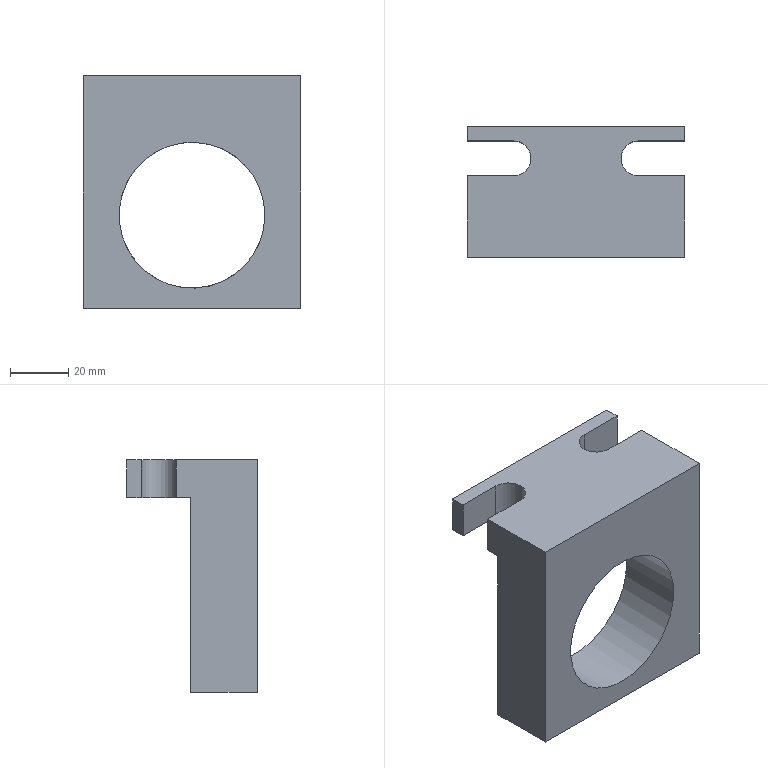Part | NX | features solid 2 | 1 solid | 17 faces | box 75 x 45 x 80 mm | volume 107465 mm3 | plane 14 | cylinder 3 | commonest cylinder face diameters 12 x2 50.2 x1
STEP:
#1=CARTESIAN_POINT('',(297.5,589.4,185.));
#2=VERTEX_POINT('',#1);
#3=CARTESIAN_POINT('',(372.5,589.4,185.));
#4=VERTEX_POINT('',#3);
#5=CARTESIAN_POINT('',(302.5,589.4,185.));
#6=DIRECTION('',(1.,0.,0.));
#7=VECTOR('',#6,1000.);
#8=LINE('',#5,#7);
#9=EDGE_CURVE('',#2,#4,#8,.T.);
#10=ORIENTED_EDGE('',*,*,#9,.F.);
#11=CARTESIAN_POINT('',(297.5,594.4,185.));
#12=VERTEX_POINT('',#11);
#13=CARTESIAN_POINT('',(297.5,565.9,185.));
#14=DIRECTION('',(0.,-1.,0.));
#15=VECTOR('',#14,1000.);
#16=LINE('',#13,#15);
#17=EDGE_CURVE('',#2,#12,#16,.F.);
#18=ORIENTED_EDGE('',*,*,#17,.T.);
#19=CARTESIAN_POINT('',(313.5,594.4,185.));
#20=VERTEX_POINT('',#19);
#21=CARTESIAN_POINT('',(302.5,594.4,185.));
#22=DIRECTION('',(-1.,0.,0.));
#23=VECTOR('',#22,1000.);
#24=LINE('',#21,#23);
#25=EDGE_CURVE('',#12,#20,#24,.F.);
#26=ORIENTED_EDGE('',*,*,#25,.T.);
#27=CARTESIAN_POINT('',(313.5,606.4,185.));
#28=VERTEX_POINT('',#27);
#29=CARTESIAN_POINT('',(313.5,600.4,185.));
#30=DIRECTION('',(0.,0.,-1.));
#31=DIRECTION('',(-1.,0.,0.));
#32=AXIS2_PLACEMENT_3D('',#29,#30,#31);
#33=CIRCLE('',#32,6.);
#34=EDGE_CURVE('',#28,#20,#33,.T.);
#35=ORIENTED_EDGE('',*,*,#34,.F.);
#36=CARTESIAN_POINT('',(297.5,606.4,185.));
#37=VERTEX_POINT('',#36);
#38=CARTESIAN_POINT('',(302.5,606.4,185.));
#39=DIRECTION('',(-1.,0.,0.));
#40=VECTOR('',#39,1000.);
#41=LINE('',#38,#40);
#42=EDGE_CURVE('',#37,#28,#41,.F.);
#43=ORIENTED_EDGE('',*,*,#42,.F.);
#44=CARTESIAN_POINT('',(297.5,611.4,185.));
#45=VERTEX_POINT('',#44);
#46=CARTESIAN_POINT('',(297.5,565.9,185.));
#47=DIRECTION('',(0.,-1.,0.));
#48=VECTOR('',#47,1000.);
#49=LINE('',#46,#48);
#50=EDGE_CURVE('',#37,#45,#49,.F.);
#51=ORIENTED_EDGE('',*,*,#50,.T.);
#52=CARTESIAN_POINT('',(372.5,611.4,185.));
#53=VERTEX_POINT('',#52);
#54=CARTESIAN_POINT('',(302.5,611.4,185.));
#55=DIRECTION('',(-1.,0.,0.));
#56=VECTOR('',#55,1000.);
#57=LINE('',#54,#56);
#58=EDGE_CURVE('',#45,#53,#57,.F.);
#59=ORIENTED_EDGE('',*,*,#58,.T.);
#60=CARTESIAN_POINT('',(372.5,606.4,185.));
#61=VERTEX_POINT('',#60);
#62=CARTESIAN_POINT('',(372.5,565.9,185.));
#63=DIRECTION('',(0.,-1.,0.));
#64=VECTOR('',#63,1000.);
#65=LINE('',#62,#64);
#66=EDGE_CURVE('',#61,#53,#65,.F.);
#67=ORIENTED_EDGE('',*,*,#66,.F.);
#68=CARTESIAN_POINT('',(356.5,606.4,185.));
#69=VERTEX_POINT('',#68);
#70=CARTESIAN_POINT('',(302.5,606.4,185.));
#71=DIRECTION('',(1.,0.,0.));
#72=VECTOR('',#71,1000.);
#73=LINE('',#70,#72);
#74=EDGE_CURVE('',#61,#69,#73,.F.);
#75=ORIENTED_EDGE('',*,*,#74,.T.);
#76=CARTESIAN_POINT('',(356.5,594.4,185.));
#77=VERTEX_POINT('',#76);
#78=CARTESIAN_POINT('',(356.5,600.4,185.));
#79=DIRECTION('',(0.,0.,-1.));
#80=DIRECTION('',(-1.,0.,0.));
#81=AXIS2_PLACEMENT_3D('',#78,#79,#80);
#82=CIRCLE('',#81,6.);
#83=EDGE_CURVE('',#69,#77,#82,.F.);
#84=ORIENTED_EDGE('',*,*,#83,.T.);
#85=CARTESIAN_POINT('',(372.5,594.4,185.));
#86=VERTEX_POINT('',#85);
#87=CARTESIAN_POINT('',(302.5,594.4,185.));
#88=DIRECTION('',(1.,0.,0.));
#89=VECTOR('',#88,1000.);
#90=LINE('',#87,#89);
#91=EDGE_CURVE('',#86,#77,#90,.F.);
#92=ORIENTED_EDGE('',*,*,#91,.F.);
#93=CARTESIAN_POINT('',(372.5,565.9,185.));
#94=DIRECTION('',(0.,-1.,0.));
#95=VECTOR('',#94,1000.);
#96=LINE('',#93,#95);
#97=EDGE_CURVE('',#4,#86,#96,.F.);
#98=ORIENTED_EDGE('',*,*,#97,.F.);
#99=EDGE_LOOP('',(#10,#18,#26,#35,#43,#51,#59,#67,#75,#84,#92,#98));
#100=FACE_BOUND('',#99,.T.);
#101=CARTESIAN_POINT('',(302.5,565.9,185.));
#102=DIRECTION('',(0.,0.,-1.));
#103=DIRECTION('',(1.,0.,0.));
#104=AXIS2_PLACEMENT_3D('',#101,#102,#103);
#105=PLANE('',#104);
#106=ADVANCED_FACE('',(#100),#105,.T.);
#107=CARTESIAN_POINT('',(297.5,611.4,198.));
#108=VERTEX_POINT('',#107);
#109=CARTESIAN_POINT('',(372.5,611.4,198.));
#110=VERTEX_POINT('',#109);
#111=CARTESIAN_POINT('',(302.5,611.4,198.));
#112=DIRECTION('',(-1.,0.,0.));
#113=VECTOR('',#112,1000.);
#114=LINE('',#111,#113);
#115=EDGE_CURVE('',#108,#110,#114,.F.);
#116=ORIENTED_EDGE('',*,*,#115,.T.);
#117=CARTESIAN_POINT('',(372.5,611.4,190.));
#118=DIRECTION('',(0.,0.,1.));
#119=VECTOR('',#118,1000.);
#120=LINE('',#117,#119);
#121=EDGE_CURVE('',#53,#110,#120,.T.);
#122=ORIENTED_EDGE('',*,*,#121,.F.);
#123=ORIENTED_EDGE('',*,*,#58,.F.);
#124=CARTESIAN_POINT('',(297.5,611.4,190.));
#125=DIRECTION('',(0.,0.,1.));
#126=VECTOR('',#125,1000.);
#127=LINE('',#124,#126);
#128=EDGE_CURVE('',#45,#108,#127,.T.);
#129=ORIENTED_EDGE('',*,*,#128,.T.);
#130=EDGE_LOOP('',(#116,#122,#123,#129));
#131=FACE_BOUND('',#130,.T.);
#132=CARTESIAN_POINT('',(302.5,611.4,190.));
#133=DIRECTION('',(0.,-1.,0.));
#134=DIRECTION('',(1.,0.,0.));
#135=AXIS2_PLACEMENT_3D('',#132,#133,#134);
#136=PLANE('',#135);
#137=ADVANCED_FACE('',(#131),#136,.F.);
#138=CARTESIAN_POINT('',(297.5,606.4,198.));
#139=VERTEX_POINT('',#138);
#140=CARTESIAN_POINT('',(297.5,565.9,198.));
#141=DIRECTION('',(0.,-1.,0.));
#142=VECTOR('',#141,1000.);
#143=LINE('',#140,#142);
#144=EDGE_CURVE('',#139,#108,#143,.F.);
#145=ORIENTED_EDGE('',*,*,#144,.T.);
#146=ORIENTED_EDGE('',*,*,#128,.F.);
#147=ORIENTED_EDGE('',*,*,#50,.F.);
#148=CARTESIAN_POINT('',(297.5,606.4,190.));
#149=DIRECTION('',(0.,0.,1.));
#150=VECTOR('',#149,1000.);
#151=LINE('',#148,#150);
#152=EDGE_CURVE('',#37,#139,#151,.T.);
#153=ORIENTED_EDGE('',*,*,#152,.T.);
#154=EDGE_LOOP('',(#145,#146,#147,#153));
#155=FACE_BOUND('',#154,.T.);
#156=CARTESIAN_POINT('',(297.5,565.9,190.));
#157=DIRECTION('',(1.,0.,0.));
#158=DIRECTION('',(0.,1.,0.));
#159=AXIS2_PLACEMENT_3D('',#156,#157,#158);
#160=PLANE('',#159);
#161=ADVANCED_FACE('',(#155),#160,.F.);
#162=CARTESIAN_POINT('',(313.5,606.4,198.));
#163=VERTEX_POINT('',#162);
#164=CARTESIAN_POINT('',(302.5,606.4,198.));
#165=DIRECTION('',(-1.,0.,0.));
#166=VECTOR('',#165,1000.);
#167=LINE('',#164,#166);
#168=EDGE_CURVE('',#139,#163,#167,.F.);
#169=ORIENTED_EDGE('',*,*,#168,.F.);
#170=ORIENTED_EDGE('',*,*,#152,.F.);
#171=ORIENTED_EDGE('',*,*,#42,.T.);
#172=CARTESIAN_POINT('',(313.5,606.4,190.));
#173=DIRECTION('',(0.,0.,1.));
#174=VECTOR('',#173,1000.);
#175=LINE('',#172,#174);
#176=EDGE_CURVE('',#28,#163,#175,.T.);
#177=ORIENTED_EDGE('',*,*,#176,.T.);
#178=EDGE_LOOP('',(#169,#170,#171,#177));
#179=FACE_BOUND('',#178,.T.);
#180=CARTESIAN_POINT('',(367.5,606.4,190.));
#181=DIRECTION('',(0.,-1.,0.));
#182=DIRECTION('',(1.,0.,0.));
#183=AXIS2_PLACEMENT_3D('',#180,#181,#182);
#184=PLANE('',#183);
#185=ADVANCED_FACE('',(#179),#184,.T.);
#186=CARTESIAN_POINT('',(313.5,594.4,198.));
#187=VERTEX_POINT('',#186);
#188=CARTESIAN_POINT('',(313.5,600.4,198.));
#189=DIRECTION('',(0.,0.,-1.));
#190=DIRECTION('',(-1.,0.,0.));
#191=AXIS2_PLACEMENT_3D('',#188,#189,#190);
#192=CIRCLE('',#191,6.);
#193=EDGE_CURVE('',#163,#187,#192,.T.);
#194=ORIENTED_EDGE('',*,*,#193,.F.);
#195=ORIENTED_EDGE('',*,*,#176,.F.);
#196=ORIENTED_EDGE('',*,*,#34,.T.);
#197=CARTESIAN_POINT('',(313.5,594.4,190.));
#198=DIRECTION('',(0.,0.,1.));
#199=VECTOR('',#198,1000.);
#200=LINE('',#197,#199);
#201=EDGE_CURVE('',#20,#187,#200,.T.);
#202=ORIENTED_EDGE('',*,*,#201,.T.);
#203=EDGE_LOOP('',(#194,#195,#196,#202));
#204=FACE_BOUND('',#203,.T.);
#205=CARTESIAN_POINT('',(313.5,600.4,190.));
#206=DIRECTION('',(0.,0.,1.));
#207=DIRECTION('',(0.,-1.,0.));
#208=AXIS2_PLACEMENT_3D('',#205,#206,#207);
#209=CYLINDRICAL_SURFACE('',#208,6.);
#210=ADVANCED_FACE('',(#204),#209,.F.);
#211=CARTESIAN_POINT('',(297.5,594.4,198.));
#212=VERTEX_POINT('',#211);
#213=CARTESIAN_POINT('',(302.5,594.4,198.));
#214=DIRECTION('',(-1.,0.,0.));
#215=VECTOR('',#214,1000.);
#216=LINE('',#213,#215);
#217=EDGE_CURVE('',#212,#187,#216,.F.);
#218=ORIENTED_EDGE('',*,*,#217,.T.);
#219=ORIENTED_EDGE('',*,*,#201,.F.);
#220=ORIENTED_EDGE('',*,*,#25,.F.);
#221=CARTESIAN_POINT('',(297.5,594.4,190.));
#222=DIRECTION('',(0.,0.,1.));
#223=VECTOR('',#222,1000.);
#224=LINE('',#221,#223);
#225=EDGE_CURVE('',#12,#212,#224,.T.);
#226=ORIENTED_EDGE('',*,*,#225,.T.);
#227=EDGE_LOOP('',(#218,#219,#220,#226));
#228=FACE_BOUND('',#227,.T.);
#229=CARTESIAN_POINT('',(367.5,594.4,190.));
#230=DIRECTION('',(0.,-1.,0.));
#231=DIRECTION('',(1.,0.,0.));
#232=AXIS2_PLACEMENT_3D('',#229,#230,#231);
#233=PLANE('',#232);
#234=ADVANCED_FACE('',(#228),#233,.F.);
#235=CARTESIAN_POINT('',(297.5,566.4,198.));
#236=VERTEX_POINT('',#235);
#237=CARTESIAN_POINT('',(297.5,565.9,198.));
#238=DIRECTION('',(0.,-1.,0.));
#239=VECTOR('',#238,1000.);
#240=LINE('',#237,#239);
#241=EDGE_CURVE('',#236,#212,#240,.F.);
#242=ORIENTED_EDGE('',*,*,#241,.T.);
#243=ORIENTED_EDGE('',*,*,#225,.F.);
#244=ORIENTED_EDGE('',*,*,#17,.F.);
#245=CARTESIAN_POINT('',(297.5,589.4,118.));
#246=VERTEX_POINT('',#245);
#247=CARTESIAN_POINT('',(297.5,589.4,150.));
#248=DIRECTION('',(0.,0.,-1.));
#249=VECTOR('',#248,1000.);
#250=LINE('',#247,#249);
#251=EDGE_CURVE('',#246,#2,#250,.F.);
#252=ORIENTED_EDGE('',*,*,#251,.F.);
#253=CARTESIAN_POINT('',(297.5,566.4,118.));
#254=VERTEX_POINT('',#253);
#255=CARTESIAN_POINT('',(297.5,565.9,118.));
#256=DIRECTION('',(0.,1.,0.));
#257=VECTOR('',#256,1000.);
#258=LINE('',#255,#257);
#259=EDGE_CURVE('',#254,#246,#258,.T.);
#260=ORIENTED_EDGE('',*,*,#259,.F.);
#261=CARTESIAN_POINT('',(297.5,566.4,190.));
#262=DIRECTION('',(0.,0.,1.));
#263=VECTOR('',#262,1000.);
#264=LINE('',#261,#263);
#265=EDGE_CURVE('',#254,#236,#264,.T.);
#266=ORIENTED_EDGE('',*,*,#265,.T.);
#267=EDGE_LOOP('',(#242,#243,#244,#252,#260,#266));
#268=FACE_BOUND('',#267,.T.);
#269=CARTESIAN_POINT('',(297.5,565.9,190.));
#270=DIRECTION('',(1.,0.,0.));
#271=DIRECTION('',(0.,1.,0.));
#272=AXIS2_PLACEMENT_3D('',#269,#270,#271);
#273=PLANE('',#272);
#274=ADVANCED_FACE('',(#268),#273,.F.);
#275=CARTESIAN_POINT('',(372.5,566.4,198.));
#276=VERTEX_POINT('',#275);
#277=CARTESIAN_POINT('',(302.5,566.4,198.));
#278=DIRECTION('',(-1.,0.,0.));
#279=VECTOR('',#278,1000.);
#280=LINE('',#277,#279);
#281=EDGE_CURVE('',#236,#276,#280,.F.);
#282=ORIENTED_EDGE('',*,*,#281,.F.);
#283=ORIENTED_EDGE('',*,*,#265,.F.);
#284=CARTESIAN_POINT('',(372.5,566.4,118.));
#285=VERTEX_POINT('',#284);
#286=CARTESIAN_POINT('',(302.5,566.4,118.));
#287=DIRECTION('',(1.,0.,0.));
#288=VECTOR('',#287,1000.);
#289=LINE('',#286,#288);
#290=EDGE_CURVE('',#254,#285,#289,.T.);
#291=ORIENTED_EDGE('',*,*,#290,.T.);
#292=CARTESIAN_POINT('',(372.5,566.4,190.));
#293=DIRECTION('',(0.,0.,1.));
#294=VECTOR('',#293,1000.);
#295=LINE('',#292,#294);
#296=EDGE_CURVE('',#285,#276,#295,.T.);
#297=ORIENTED_EDGE('',*,*,#296,.T.);
#298=EDGE_LOOP('',(#282,#283,#291,#297));
#299=FACE_BOUND('',#298,.T.);
#300=CARTESIAN_POINT('',(360.1,566.4,150.));
#301=VERTEX_POINT('',#300);
#302=CARTESIAN_POINT('',(335.,566.4,150.));
#303=DIRECTION('',(0.,-1.,0.));
#304=DIRECTION('',(1.,0.,0.));
#305=AXIS2_PLACEMENT_3D('',#302,#303,#304);
#306=CIRCLE('',#305,25.1);
#307=EDGE_CURVE('',#301,#301,#306,.T.);
#308=ORIENTED_EDGE('',*,*,#307,.F.);
#309=EDGE_LOOP('',(#308));
#310=FACE_BOUND('',#309,.T.);
#311=CARTESIAN_POINT('',(302.5,566.4,190.));
#312=DIRECTION('',(0.,-1.,0.));
#313=DIRECTION('',(1.,0.,0.));
#314=AXIS2_PLACEMENT_3D('',#311,#312,#313);
#315=PLANE('',#314);
#316=ADVANCED_FACE('',(#299,#310),#315,.T.);
#317=CARTESIAN_POINT('',(372.5,594.4,198.));
#318=VERTEX_POINT('',#317);
#319=CARTESIAN_POINT('',(372.5,565.9,198.));
#320=DIRECTION('',(0.,-1.,0.));
#321=VECTOR('',#320,1000.);
#322=LINE('',#319,#321);
#323=EDGE_CURVE('',#276,#318,#322,.F.);
#324=ORIENTED_EDGE('',*,*,#323,.F.);
#325=ORIENTED_EDGE('',*,*,#296,.F.);
#326=CARTESIAN_POINT('',(372.5,589.4,118.));
#327=VERTEX_POINT('',#326);
#328=CARTESIAN_POINT('',(372.5,565.9,118.));
#329=DIRECTION('',(0.,1.,0.));
#330=VECTOR('',#329,1000.);
#331=LINE('',#328,#330);
#332=EDGE_CURVE('',#285,#327,#331,.T.);
#333=ORIENTED_EDGE('',*,*,#332,.T.);
#334=CARTESIAN_POINT('',(372.5,589.4,150.));
#335=DIRECTION('',(0.,0.,-1.));
#336=VECTOR('',#335,1000.);
#337=LINE('',#334,#336);
#338=EDGE_CURVE('',#327,#4,#337,.F.);
#339=ORIENTED_EDGE('',*,*,#338,.T.);
#340=ORIENTED_EDGE('',*,*,#97,.T.);
#341=CARTESIAN_POINT('',(372.5,594.4,190.));
#342=DIRECTION('',(0.,0.,1.));
#343=VECTOR('',#342,1000.);
#344=LINE('',#341,#343);
#345=EDGE_CURVE('',#86,#318,#344,.T.);
#346=ORIENTED_EDGE('',*,*,#345,.T.);
#347=EDGE_LOOP('',(#324,#325,#333,#339,#340,#346));
#348=FACE_BOUND('',#347,.T.);
#349=CARTESIAN_POINT('',(372.5,565.9,190.));
#350=DIRECTION('',(1.,0.,0.));
#351=DIRECTION('',(0.,1.,0.));
#352=AXIS2_PLACEMENT_3D('',#349,#350,#351);
#353=PLANE('',#352);
#354=ADVANCED_FACE('',(#348),#353,.T.);
#355=CARTESIAN_POINT('',(356.5,594.4,198.));
#356=VERTEX_POINT('',#355);
#357=CARTESIAN_POINT('',(302.5,594.4,198.));
#358=DIRECTION('',(1.,0.,0.));
#359=VECTOR('',#358,1000.);
#360=LINE('',#357,#359);
#361=EDGE_CURVE('',#318,#356,#360,.F.);
#362=ORIENTED_EDGE('',*,*,#361,.F.);
#363=ORIENTED_EDGE('',*,*,#345,.F.);
#364=ORIENTED_EDGE('',*,*,#91,.T.);
#365=CARTESIAN_POINT('',(356.5,594.4,190.));
#366=DIRECTION('',(0.,0.,1.));
#367=VECTOR('',#366,1000.);
#368=LINE('',#365,#367);
#369=EDGE_CURVE('',#77,#356,#368,.T.);
#370=ORIENTED_EDGE('',*,*,#369,.T.);
#371=EDGE_LOOP('',(#362,#363,#364,#370));
#372=FACE_BOUND('',#371,.T.);
#373=CARTESIAN_POINT('',(302.5,594.4,190.));
#374=DIRECTION('',(0.,1.,0.));
#375=DIRECTION('',(-1.,0.,0.));
#376=AXIS2_PLACEMENT_3D('',#373,#374,#375);
#377=PLANE('',#376);
#378=ADVANCED_FACE('',(#372),#377,.T.);
#379=CARTESIAN_POINT('',(356.5,606.4,198.));
#380=VERTEX_POINT('',#379);
#381=CARTESIAN_POINT('',(356.5,600.4,198.));
#382=DIRECTION('',(0.,0.,-1.));
#383=DIRECTION('',(-1.,0.,0.));
#384=AXIS2_PLACEMENT_3D('',#381,#382,#383);
#385=CIRCLE('',#384,6.);
#386=EDGE_CURVE('',#380,#356,#385,.F.);
#387=ORIENTED_EDGE('',*,*,#386,.T.);
#388=ORIENTED_EDGE('',*,*,#369,.F.);
#389=ORIENTED_EDGE('',*,*,#83,.F.);
#390=CARTESIAN_POINT('',(356.5,606.4,190.));
#391=DIRECTION('',(0.,0.,1.));
#392=VECTOR('',#391,1000.);
#393=LINE('',#390,#392);
#394=EDGE_CURVE('',#69,#380,#393,.T.);
#395=ORIENTED_EDGE('',*,*,#394,.T.);
#396=EDGE_LOOP('',(#387,#388,#389,#395));
#397=FACE_BOUND('',#396,.T.);
#398=CARTESIAN_POINT('',(356.5,600.4,190.));
#399=DIRECTION('',(0.,0.,1.));
#400=DIRECTION('',(0.,-1.,0.));
#401=AXIS2_PLACEMENT_3D('',#398,#399,#400);
#402=CYLINDRICAL_SURFACE('',#401,6.);
#403=ADVANCED_FACE('',(#397),#402,.F.);
#404=CARTESIAN_POINT('',(372.5,606.4,198.));
#405=VERTEX_POINT('',#404);
#406=CARTESIAN_POINT('',(302.5,606.4,198.));
#407=DIRECTION('',(1.,0.,0.));
#408=VECTOR('',#407,1000.);
#409=LINE('',#406,#408);
#410=EDGE_CURVE('',#405,#380,#409,.F.);
#411=ORIENTED_EDGE('',*,*,#410,.T.);
#412=ORIENTED_EDGE('',*,*,#394,.F.);
#413=ORIENTED_EDGE('',*,*,#74,.F.);
#414=CARTESIAN_POINT('',(372.5,606.4,190.));
#415=DIRECTION('',(0.,0.,1.));
#416=VECTOR('',#415,1000.);
#417=LINE('',#414,#416);
#418=EDGE_CURVE('',#61,#405,#417,.T.);
#419=ORIENTED_EDGE('',*,*,#418,.T.);
#420=EDGE_LOOP('',(#411,#412,#413,#419));
#421=FACE_BOUND('',#420,.T.);
#422=CARTESIAN_POINT('',(302.5,606.4,190.));
#423=DIRECTION('',(0.,1.,0.));
#424=DIRECTION('',(-1.,0.,0.));
#425=AXIS2_PLACEMENT_3D('',#422,#423,#424);
#426=PLANE('',#425);
#427=ADVANCED_FACE('',(#421),#426,.F.);
#428=CARTESIAN_POINT('',(372.5,565.9,198.));
#429=DIRECTION('',(0.,-1.,0.));
#430=VECTOR('',#429,1000.);
#431=LINE('',#428,#430);
#432=EDGE_CURVE('',#405,#110,#431,.F.);
#433=ORIENTED_EDGE('',*,*,#432,.F.);
#434=ORIENTED_EDGE('',*,*,#418,.F.);
#435=ORIENTED_EDGE('',*,*,#66,.T.);
#436=ORIENTED_EDGE('',*,*,#121,.T.);
#437=EDGE_LOOP('',(#433,#434,#435,#436));
#438=FACE_BOUND('',#437,.T.);
#439=CARTESIAN_POINT('',(372.5,565.9,190.));
#440=DIRECTION('',(1.,0.,0.));
#441=DIRECTION('',(0.,1.,0.));
#442=AXIS2_PLACEMENT_3D('',#439,#440,#441);
#443=PLANE('',#442);
#444=ADVANCED_FACE('',(#438),#443,.T.);
#445=ORIENTED_EDGE('',*,*,#115,.F.);
#446=ORIENTED_EDGE('',*,*,#144,.F.);
#447=ORIENTED_EDGE('',*,*,#168,.T.);
#448=ORIENTED_EDGE('',*,*,#193,.T.);
#449=ORIENTED_EDGE('',*,*,#217,.F.);
#450=ORIENTED_EDGE('',*,*,#241,.F.);
#451=ORIENTED_EDGE('',*,*,#281,.T.);
#452=ORIENTED_EDGE('',*,*,#323,.T.);
#453=ORIENTED_EDGE('',*,*,#361,.T.);
#454=ORIENTED_EDGE('',*,*,#386,.F.);
#455=ORIENTED_EDGE('',*,*,#410,.F.);
#456=ORIENTED_EDGE('',*,*,#432,.T.);
#457=EDGE_LOOP('',(#445,#446,#447,#448,#449,#450,#451,#452,#453,#454,#455,#456));
#458=FACE_BOUND('',#457,.T.);
#459=CARTESIAN_POINT('',(302.5,565.9,198.));
#460=DIRECTION('',(0.,0.,-1.));
#461=DIRECTION('',(1.,0.,0.));
#462=AXIS2_PLACEMENT_3D('',#459,#460,#461);
#463=PLANE('',#462);
#464=ADVANCED_FACE('',(#458),#463,.F.);
#465=ORIENTED_EDGE('',*,*,#290,.F.);
#466=ORIENTED_EDGE('',*,*,#259,.T.);
#467=CARTESIAN_POINT('',(335.,589.4,118.));
#468=DIRECTION('',(-1.,0.,0.));
#469=VECTOR('',#468,1000.);
#470=LINE('',#467,#469);
#471=EDGE_CURVE('',#246,#327,#470,.F.);
#472=ORIENTED_EDGE('',*,*,#471,.T.);
#473=ORIENTED_EDGE('',*,*,#332,.F.);
#474=EDGE_LOOP('',(#465,#466,#472,#473));
#475=FACE_BOUND('',#474,.T.);
#476=CARTESIAN_POINT('',(302.5,565.9,118.));
#477=DIRECTION('',(0.,0.,-1.));
#478=DIRECTION('',(1.,0.,0.));
#479=AXIS2_PLACEMENT_3D('',#476,#477,#478);
#480=PLANE('',#479);
#481=ADVANCED_FACE('',(#475),#480,.T.);
#482=CARTESIAN_POINT('',(309.9,589.4,150.));
#483=VERTEX_POINT('',#482);
#484=CARTESIAN_POINT('',(335.,589.4,150.));
#485=DIRECTION('',(0.,1.,0.));
#486=DIRECTION('',(-1.,0.,0.));
#487=AXIS2_PLACEMENT_3D('',#484,#485,#486);
#488=CIRCLE('',#487,25.1);
#489=EDGE_CURVE('',#483,#483,#488,.F.);
#490=ORIENTED_EDGE('',*,*,#489,.T.);
#491=EDGE_LOOP('',(#490));
#492=FACE_BOUND('',#491,.T.);
#493=ORIENTED_EDGE('',*,*,#9,.T.);
#494=ORIENTED_EDGE('',*,*,#338,.F.);
#495=ORIENTED_EDGE('',*,*,#471,.F.);
#496=ORIENTED_EDGE('',*,*,#251,.T.);
#497=EDGE_LOOP('',(#493,#494,#495,#496));
#498=FACE_BOUND('',#497,.T.);
#499=CARTESIAN_POINT('',(335.,589.4,150.));
#500=DIRECTION('',(0.,1.,0.));
#501=DIRECTION('',(0.,0.,-1.));
#502=AXIS2_PLACEMENT_3D('',#499,#500,#501);
#503=PLANE('',#502);
#504=ADVANCED_FACE('',(#492,#498),#503,.T.);
#505=ORIENTED_EDGE('',*,*,#307,.T.);
#506=EDGE_LOOP('',(#505));
#507=FACE_BOUND('',#506,.T.);
#508=ORIENTED_EDGE('',*,*,#489,.F.);
#509=EDGE_LOOP('',(#508));
#510=FACE_BOUND('',#509,.T.);
#511=CARTESIAN_POINT('',(335.,603.,150.));
#512=DIRECTION('',(0.,-1.,0.));
#513=DIRECTION('',(1.,0.,0.));
#514=AXIS2_PLACEMENT_3D('',#511,#512,#513);
#515=CYLINDRICAL_SURFACE('',#514,25.1);
#516=ADVANCED_FACE('',(#507,#510),#515,.F.);
#517=CLOSED_SHELL('',(#106,#137,#161,#185,#210,#234,#274,#316,#354,#378,#403,#427,#444,#464,#481,#504,#516));
#518=MANIFOLD_SOLID_BREP('',#517);
#519=(LENGTH_UNIT()NAMED_UNIT(*)SI_UNIT(.MILLI.,.METRE.));
#520=UNCERTAINTY_MEASURE_WITH_UNIT(LENGTH_MEASURE(0.00001),#519,'','');
#521=(NAMED_UNIT(*)PLANE_ANGLE_UNIT()SI_UNIT($,.RADIAN.));
#522=(NAMED_UNIT(*)SI_UNIT($,.STERADIAN.)SOLID_ANGLE_UNIT());
#523=(GEOMETRIC_REPRESENTATION_CONTEXT(3)GLOBAL_UNCERTAINTY_ASSIGNED_CONTEXT((#520))GLOBAL_UNIT_ASSIGNED_CONTEXT((#519,#521,#522))REPRESENTATION_CONTEXT('',''));
#524=ADVANCED_BREP_SHAPE_REPRESENTATION('',(#518),#523);